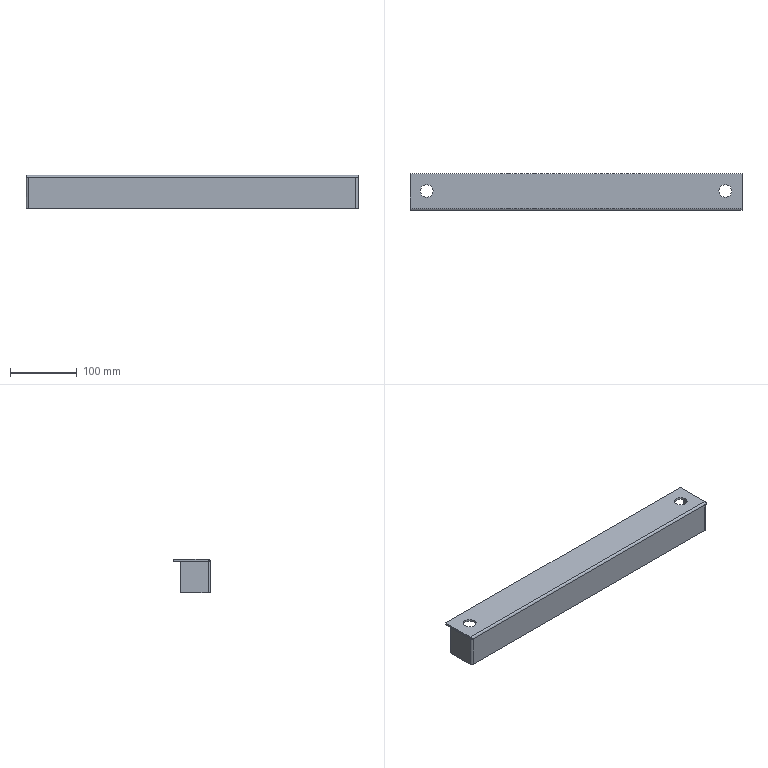Part | STEP file | 1 solid | 36 faces | box 498 x 55 x 50 mm | volume 161185 mm3 | plane 26 | cylinder 10 | commonest cylinder face diameters 19 x4 0.4 x3 6.4 x3